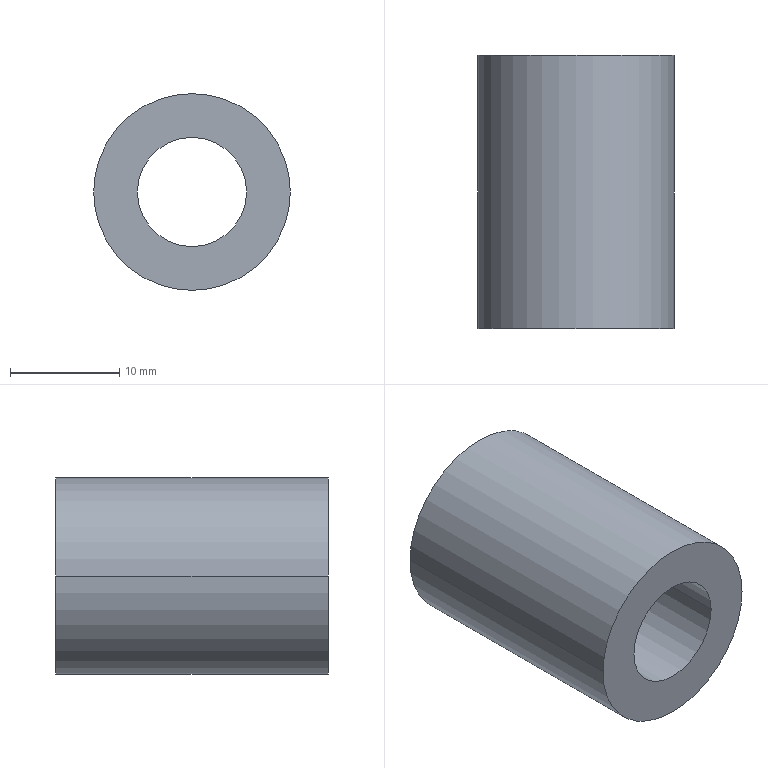Part | SolidWorks | features Revolution 1 | 1 solid | 6 faces | box 18 x 25 x 18 mm | volume 4398 mm3 | cylinder 4 | plane 2 | commonest cylinder face diameters 10 x2 18 x2
STEP:
#1=CARTESIAN_POINT('',(9.,25.,0.));
#2=VERTEX_POINT('',#1);
#3=CARTESIAN_POINT('',(-9.,25.,0.));
#4=VERTEX_POINT('',#3);
#5=CARTESIAN_POINT('',(0.,25.,0.));
#6=DIRECTION('',(0.,-1.,0.));
#7=DIRECTION('',(1.,0.,0.));
#8=AXIS2_PLACEMENT_3D('',#5,#6,#7);
#9=CIRCLE('',#8,9.);
#10=EDGE_CURVE('',#2,#4,#9,.T.);
#11=ORIENTED_EDGE('',*,*,#10,.T.);
#12=CARTESIAN_POINT('',(-9.,0.,0.));
#13=VERTEX_POINT('',#12);
#14=CARTESIAN_POINT('',(-9.,-309.732,0.));
#15=DIRECTION('',(0.,-1.,0.));
#16=VECTOR('',#15,1000.);
#17=LINE('',#14,#16);
#18=EDGE_CURVE('',#4,#13,#17,.T.);
#19=ORIENTED_EDGE('',*,*,#18,.T.);
#20=CARTESIAN_POINT('',(9.,0.,0.));
#21=VERTEX_POINT('',#20);
#22=CARTESIAN_POINT('',(0.,0.,0.));
#23=DIRECTION('',(0.,-1.,0.));
#24=DIRECTION('',(1.,0.,0.));
#25=AXIS2_PLACEMENT_3D('',#22,#23,#24);
#26=CIRCLE('',#25,9.);
#27=EDGE_CURVE('',#21,#13,#26,.T.);
#28=ORIENTED_EDGE('',*,*,#27,.F.);
#29=CARTESIAN_POINT('',(9.,-309.732,0.));
#30=DIRECTION('',(0.,-1.,0.));
#31=VECTOR('',#30,1000.);
#32=LINE('',#29,#31);
#33=EDGE_CURVE('',#2,#21,#32,.T.);
#34=ORIENTED_EDGE('',*,*,#33,.F.);
#35=EDGE_LOOP('',(#11,#19,#28,#34));
#36=FACE_OUTER_BOUND('',#35,.T.);
#37=CARTESIAN_POINT('',(0.,-309.732,0.));
#38=DIRECTION('',(0.,-1.,0.));
#39=DIRECTION('',(1.,0.,0.));
#40=AXIS2_PLACEMENT_3D('',#37,#38,#39);
#41=CYLINDRICAL_SURFACE('',#40,9.);
#42=ADVANCED_FACE('',(#36),#41,.T.);
#43=CARTESIAN_POINT('',(-5.,25.,0.));
#44=VERTEX_POINT('',#43);
#45=CARTESIAN_POINT('',(5.,25.,0.));
#46=VERTEX_POINT('',#45);
#47=CARTESIAN_POINT('',(0.,25.,0.));
#48=DIRECTION('',(0.,-1.,0.));
#49=DIRECTION('',(1.,0.,0.));
#50=AXIS2_PLACEMENT_3D('',#47,#48,#49);
#51=CIRCLE('',#50,5.);
#52=EDGE_CURVE('',#44,#46,#51,.T.);
#53=ORIENTED_EDGE('',*,*,#52,.F.);
#54=CARTESIAN_POINT('',(-5.,0.,0.));
#55=VERTEX_POINT('',#54);
#56=CARTESIAN_POINT('',(-5.,-309.732,0.));
#57=DIRECTION('',(0.,-1.,0.));
#58=VECTOR('',#57,1000.);
#59=LINE('',#56,#58);
#60=EDGE_CURVE('',#44,#55,#59,.T.);
#61=ORIENTED_EDGE('',*,*,#60,.T.);
#62=CARTESIAN_POINT('',(5.,0.,0.));
#63=VERTEX_POINT('',#62);
#64=CARTESIAN_POINT('',(0.,0.,0.));
#65=DIRECTION('',(0.,-1.,0.));
#66=DIRECTION('',(1.,0.,0.));
#67=AXIS2_PLACEMENT_3D('',#64,#65,#66);
#68=CIRCLE('',#67,5.);
#69=EDGE_CURVE('',#55,#63,#68,.T.);
#70=ORIENTED_EDGE('',*,*,#69,.T.);
#71=CARTESIAN_POINT('',(5.,-309.732,0.));
#72=DIRECTION('',(0.,-1.,0.));
#73=VECTOR('',#72,1000.);
#74=LINE('',#71,#73);
#75=EDGE_CURVE('',#46,#63,#74,.T.);
#76=ORIENTED_EDGE('',*,*,#75,.F.);
#77=EDGE_LOOP('',(#53,#61,#70,#76));
#78=FACE_OUTER_BOUND('',#77,.T.);
#79=CARTESIAN_POINT('',(0.,-309.732,0.));
#80=DIRECTION('',(0.,-1.,0.));
#81=DIRECTION('',(1.,0.,0.));
#82=AXIS2_PLACEMENT_3D('',#79,#80,#81);
#83=CYLINDRICAL_SURFACE('',#82,5.);
#84=ADVANCED_FACE('',(#78),#83,.F.);
#85=ORIENTED_EDGE('',*,*,#60,.F.);
#86=CARTESIAN_POINT('',(0.,25.,0.));
#87=DIRECTION('',(0.,-1.,0.));
#88=DIRECTION('',(1.,0.,0.));
#89=AXIS2_PLACEMENT_3D('',#86,#87,#88);
#90=CIRCLE('',#89,5.);
#91=EDGE_CURVE('',#46,#44,#90,.T.);
#92=ORIENTED_EDGE('',*,*,#91,.F.);
#93=ORIENTED_EDGE('',*,*,#75,.T.);
#94=CARTESIAN_POINT('',(0.,0.,0.));
#95=DIRECTION('',(0.,-1.,0.));
#96=DIRECTION('',(1.,0.,0.));
#97=AXIS2_PLACEMENT_3D('',#94,#95,#96);
#98=CIRCLE('',#97,5.);
#99=EDGE_CURVE('',#63,#55,#98,.T.);
#100=ORIENTED_EDGE('',*,*,#99,.T.);
#101=EDGE_LOOP('',(#85,#92,#93,#100));
#102=FACE_OUTER_BOUND('',#101,.T.);
#103=CARTESIAN_POINT('',(0.,-309.732,0.));
#104=DIRECTION('',(0.,-1.,0.));
#105=DIRECTION('',(1.,0.,0.));
#106=AXIS2_PLACEMENT_3D('',#103,#104,#105);
#107=CYLINDRICAL_SURFACE('',#106,5.);
#108=ADVANCED_FACE('',(#102),#107,.F.);
#109=ORIENTED_EDGE('',*,*,#27,.T.);
#110=CARTESIAN_POINT('',(0.,0.,0.));
#111=DIRECTION('',(0.,-1.,0.));
#112=DIRECTION('',(1.,0.,0.));
#113=AXIS2_PLACEMENT_3D('',#110,#111,#112);
#114=CIRCLE('',#113,9.);
#115=EDGE_CURVE('',#13,#21,#114,.T.);
#116=ORIENTED_EDGE('',*,*,#115,.T.);
#117=EDGE_LOOP('',(#109,#116));
#118=FACE_OUTER_BOUND('',#117,.T.);
#119=ORIENTED_EDGE('',*,*,#99,.F.);
#120=ORIENTED_EDGE('',*,*,#69,.F.);
#121=EDGE_LOOP('',(#119,#120));
#122=FACE_BOUND('',#121,.T.);
#123=CARTESIAN_POINT('',(5.,0.,0.));
#124=DIRECTION('',(0.,-1.,0.));
#125=DIRECTION('',(1.,0.,0.));
#126=AXIS2_PLACEMENT_3D('',#123,#124,#125);
#127=PLANE('',#126);
#128=ADVANCED_FACE('',(#118,#122),#127,.T.);
#129=ORIENTED_EDGE('',*,*,#18,.F.);
#130=CARTESIAN_POINT('',(0.,25.,0.));
#131=DIRECTION('',(0.,-1.,0.));
#132=DIRECTION('',(1.,0.,0.));
#133=AXIS2_PLACEMENT_3D('',#130,#131,#132);
#134=CIRCLE('',#133,9.);
#135=EDGE_CURVE('',#4,#2,#134,.T.);
#136=ORIENTED_EDGE('',*,*,#135,.T.);
#137=ORIENTED_EDGE('',*,*,#33,.T.);
#138=ORIENTED_EDGE('',*,*,#115,.F.);
#139=EDGE_LOOP('',(#129,#136,#137,#138));
#140=FACE_OUTER_BOUND('',#139,.T.);
#141=CARTESIAN_POINT('',(0.,-309.732,0.));
#142=DIRECTION('',(0.,-1.,0.));
#143=DIRECTION('',(1.,0.,0.));
#144=AXIS2_PLACEMENT_3D('',#141,#142,#143);
#145=CYLINDRICAL_SURFACE('',#144,9.);
#146=ADVANCED_FACE('',(#140),#145,.T.);
#147=ORIENTED_EDGE('',*,*,#91,.T.);
#148=ORIENTED_EDGE('',*,*,#52,.T.);
#149=EDGE_LOOP('',(#147,#148));
#150=FACE_BOUND('',#149,.T.);
#151=ORIENTED_EDGE('',*,*,#10,.F.);
#152=ORIENTED_EDGE('',*,*,#135,.F.);
#153=EDGE_LOOP('',(#151,#152));
#154=FACE_OUTER_BOUND('',#153,.T.);
#155=CARTESIAN_POINT('',(5.,25.,0.));
#156=DIRECTION('',(0.,1.,0.));
#157=DIRECTION('',(-1.,0.,0.));
#158=AXIS2_PLACEMENT_3D('',#155,#156,#157);
#159=PLANE('',#158);
#160=ADVANCED_FACE('',(#150,#154),#159,.T.);
#161=CLOSED_SHELL('',(#42,#84,#108,#128,#146,#160));
#162=MANIFOLD_SOLID_BREP('',#161);
#163=CARTESIAN_POINT('',(0.,0.,0.));
#164=DIRECTION('',(0.,0.,1.));
#165=DIRECTION('',(1.,0.,0.));
#166=AXIS2_PLACEMENT_3D('',#163,#164,#165);
#167=(LENGTH_UNIT()NAMED_UNIT(*)SI_UNIT(.MILLI.,.METRE.));
#168=UNCERTAINTY_MEASURE_WITH_UNIT(LENGTH_MEASURE(0.00001),#167,'','');
#169=(NAMED_UNIT(*)PLANE_ANGLE_UNIT()SI_UNIT($,.RADIAN.));
#170=(NAMED_UNIT(*)SI_UNIT($,.STERADIAN.)SOLID_ANGLE_UNIT());
#171=(GEOMETRIC_REPRESENTATION_CONTEXT(3)GLOBAL_UNCERTAINTY_ASSIGNED_CONTEXT((#168))GLOBAL_UNIT_ASSIGNED_CONTEXT((#167,#169,#170))REPRESENTATION_CONTEXT('',''));
#172=ADVANCED_BREP_SHAPE_REPRESENTATION('',(#162,#166),#171);